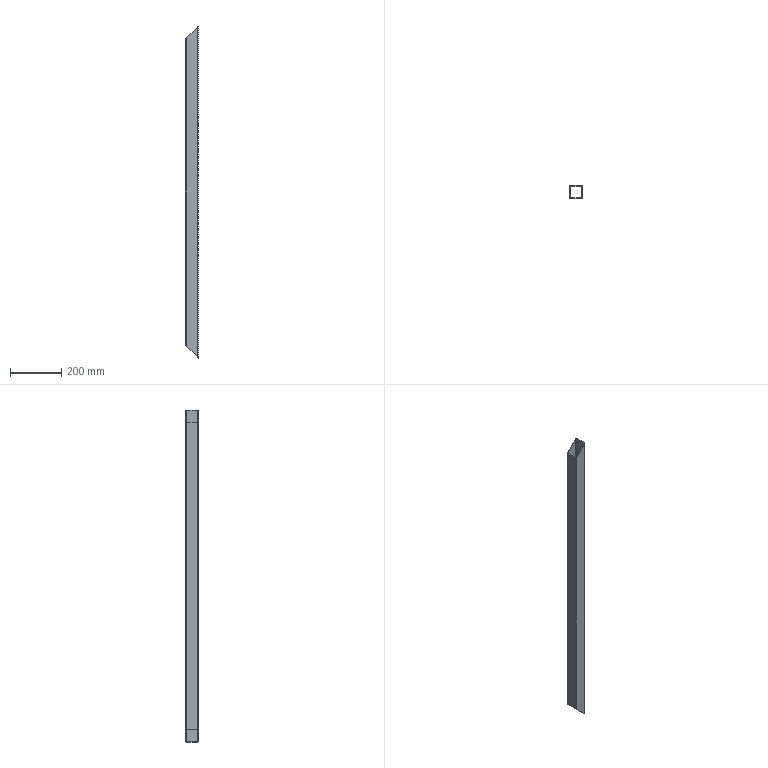Part | SolidWorks | features BaseBody 1 | 1 solid | 18 faces | box 50 x 50 x 1296 mm | volume 465629 mm3 | plane 10 | cylinder 8 | commonest cylinder face diameters 4 x4 8 x4
STEP:
#1=CARTESIAN_POINT('',(-23.,21.,600.));
#2=VERTEX_POINT('',#1);
#3=CARTESIAN_POINT('',(-23.,-21.,600.));
#4=VERTEX_POINT('',#3);
#5=CARTESIAN_POINT('',(-23.,21.,600.));
#6=DIRECTION('',(0.,-1.,0.));
#7=VECTOR('',#6,1000.);
#8=LINE('',#5,#7);
#9=EDGE_CURVE('',#2,#4,#8,.T.);
#10=ORIENTED_EDGE('',*,*,#9,.F.);
#11=CARTESIAN_POINT('',(-21.,23.,602.));
#12=VERTEX_POINT('',#11);
#13=CARTESIAN_POINT('',(-21.,23.,602.));
#14=CARTESIAN_POINT('',(-22.172,23.,600.828));
#15=CARTESIAN_POINT('',(-23.,22.172,600.));
#16=CARTESIAN_POINT('',(-23.,21.,600.));
#17=(BOUNDED_CURVE()B_SPLINE_CURVE(3,(#13,#14,#15,#16),.UNSPECIFIED.,.F.,.F.)B_SPLINE_CURVE_WITH_KNOTS((4,4),(4.712,6.283),.UNSPECIFIED.)CURVE()GEOMETRIC_REPRESENTATION_ITEM()RATIONAL_B_SPLINE_CURVE((1.,0.8047,0.8047,1.))REPRESENTATION_ITEM(''));
#18=EDGE_CURVE('',#12,#2,#17,.T.);
#19=ORIENTED_EDGE('',*,*,#18,.F.);
#20=CARTESIAN_POINT('',(21.,23.,644.));
#21=VERTEX_POINT('',#20);
#22=CARTESIAN_POINT('',(2.,23.,625.));
#23=DIRECTION('',(-0.7071,0.,-0.7071));
#24=VECTOR('',#23,1000.);
#25=LINE('',#22,#24);
#26=EDGE_CURVE('',#21,#12,#25,.T.);
#27=ORIENTED_EDGE('',*,*,#26,.F.);
#28=CARTESIAN_POINT('',(23.,21.,646.));
#29=VERTEX_POINT('',#28);
#30=CARTESIAN_POINT('',(23.,21.,646.));
#31=CARTESIAN_POINT('',(23.,22.172,646.));
#32=CARTESIAN_POINT('',(22.172,23.,645.172));
#33=CARTESIAN_POINT('',(21.,23.,644.));
#34=(BOUNDED_CURVE()B_SPLINE_CURVE(3,(#30,#31,#32,#33),.UNSPECIFIED.,.F.,.F.)B_SPLINE_CURVE_WITH_KNOTS((4,4),(3.142,4.712),.UNSPECIFIED.)CURVE()GEOMETRIC_REPRESENTATION_ITEM()RATIONAL_B_SPLINE_CURVE((1.,0.8047,0.8047,1.))REPRESENTATION_ITEM(''));
#35=EDGE_CURVE('',#29,#21,#34,.T.);
#36=ORIENTED_EDGE('',*,*,#35,.F.);
#37=CARTESIAN_POINT('',(23.,-21.,646.));
#38=VERTEX_POINT('',#37);
#39=CARTESIAN_POINT('',(23.,21.,646.));
#40=DIRECTION('',(0.,1.,0.));
#41=VECTOR('',#40,1000.);
#42=LINE('',#39,#41);
#43=EDGE_CURVE('',#38,#29,#42,.T.);
#44=ORIENTED_EDGE('',*,*,#43,.F.);
#45=CARTESIAN_POINT('',(21.,-23.,644.));
#46=VERTEX_POINT('',#45);
#47=CARTESIAN_POINT('',(21.,-23.,644.));
#48=CARTESIAN_POINT('',(22.172,-23.,645.172));
#49=CARTESIAN_POINT('',(23.,-22.172,646.));
#50=CARTESIAN_POINT('',(23.,-21.,646.));
#51=(BOUNDED_CURVE()B_SPLINE_CURVE(3,(#47,#48,#49,#50),.UNSPECIFIED.,.F.,.F.)B_SPLINE_CURVE_WITH_KNOTS((4,4),(1.571,3.142),.UNSPECIFIED.)CURVE()GEOMETRIC_REPRESENTATION_ITEM()RATIONAL_B_SPLINE_CURVE((1.,0.8047,0.8047,1.))REPRESENTATION_ITEM(''));
#52=EDGE_CURVE('',#46,#38,#51,.T.);
#53=ORIENTED_EDGE('',*,*,#52,.F.);
#54=CARTESIAN_POINT('',(-21.,-23.,602.));
#55=VERTEX_POINT('',#54);
#56=CARTESIAN_POINT('',(2.,-23.,625.));
#57=DIRECTION('',(0.7071,0.,0.7071));
#58=VECTOR('',#57,1000.);
#59=LINE('',#56,#58);
#60=EDGE_CURVE('',#55,#46,#59,.T.);
#61=ORIENTED_EDGE('',*,*,#60,.F.);
#62=CARTESIAN_POINT('',(-23.,-21.,600.));
#63=CARTESIAN_POINT('',(-23.,-22.172,600.));
#64=CARTESIAN_POINT('',(-22.172,-23.,600.828));
#65=CARTESIAN_POINT('',(-21.,-23.,602.));
#66=(BOUNDED_CURVE()B_SPLINE_CURVE(3,(#62,#63,#64,#65),.UNSPECIFIED.,.F.,.F.)B_SPLINE_CURVE_WITH_KNOTS((4,4),(0.,1.571),.UNSPECIFIED.)CURVE()GEOMETRIC_REPRESENTATION_ITEM()RATIONAL_B_SPLINE_CURVE((1.,0.8047,0.8047,1.))REPRESENTATION_ITEM(''));
#67=EDGE_CURVE('',#4,#55,#66,.T.);
#68=ORIENTED_EDGE('',*,*,#67,.F.);
#69=EDGE_LOOP('',(#10,#19,#27,#36,#44,#53,#61,#68));
#70=FACE_BOUND('',#69,.T.);
#71=CARTESIAN_POINT('',(-25.,-21.,598.));
#72=VERTEX_POINT('',#71);
#73=CARTESIAN_POINT('',(-21.,-25.,602.));
#74=VERTEX_POINT('',#73);
#75=CARTESIAN_POINT('',(-25.,-21.,598.));
#76=CARTESIAN_POINT('',(-25.,-23.343,598.));
#77=CARTESIAN_POINT('',(-23.343,-25.,599.657));
#78=CARTESIAN_POINT('',(-21.,-25.,602.));
#79=(BOUNDED_CURVE()B_SPLINE_CURVE(3,(#75,#76,#77,#78),.UNSPECIFIED.,.F.,.F.)B_SPLINE_CURVE_WITH_KNOTS((4,4),(0.,1.571),.UNSPECIFIED.)CURVE()GEOMETRIC_REPRESENTATION_ITEM()RATIONAL_B_SPLINE_CURVE((1.,0.8047,0.8047,1.))REPRESENTATION_ITEM(''));
#80=EDGE_CURVE('',#72,#74,#79,.T.);
#81=ORIENTED_EDGE('',*,*,#80,.T.);
#82=CARTESIAN_POINT('',(21.,-25.,644.));
#83=VERTEX_POINT('',#82);
#84=CARTESIAN_POINT('',(25.,-25.,648.));
#85=DIRECTION('',(0.7071,0.,0.7071));
#86=VECTOR('',#85,1000.);
#87=LINE('',#84,#86);
#88=EDGE_CURVE('',#74,#83,#87,.T.);
#89=ORIENTED_EDGE('',*,*,#88,.T.);
#90=CARTESIAN_POINT('',(25.,-21.,648.));
#91=VERTEX_POINT('',#90);
#92=CARTESIAN_POINT('',(21.,-25.,644.));
#93=CARTESIAN_POINT('',(23.343,-25.,646.343));
#94=CARTESIAN_POINT('',(25.,-23.343,648.));
#95=CARTESIAN_POINT('',(25.,-21.,648.));
#96=(BOUNDED_CURVE()B_SPLINE_CURVE(3,(#92,#93,#94,#95),.UNSPECIFIED.,.F.,.F.)B_SPLINE_CURVE_WITH_KNOTS((4,4),(1.571,3.142),.UNSPECIFIED.)CURVE()GEOMETRIC_REPRESENTATION_ITEM()RATIONAL_B_SPLINE_CURVE((1.,0.8047,0.8047,1.))REPRESENTATION_ITEM(''));
#97=EDGE_CURVE('',#83,#91,#96,.T.);
#98=ORIENTED_EDGE('',*,*,#97,.T.);
#99=CARTESIAN_POINT('',(25.,21.,648.));
#100=VERTEX_POINT('',#99);
#101=CARTESIAN_POINT('',(25.,21.,648.));
#102=DIRECTION('',(0.,1.,0.));
#103=VECTOR('',#102,1000.);
#104=LINE('',#101,#103);
#105=EDGE_CURVE('',#91,#100,#104,.T.);
#106=ORIENTED_EDGE('',*,*,#105,.T.);
#107=CARTESIAN_POINT('',(21.,25.,644.));
#108=VERTEX_POINT('',#107);
#109=CARTESIAN_POINT('',(25.,21.,648.));
#110=CARTESIAN_POINT('',(25.,23.343,648.));
#111=CARTESIAN_POINT('',(23.343,25.,646.343));
#112=CARTESIAN_POINT('',(21.,25.,644.));
#113=(BOUNDED_CURVE()B_SPLINE_CURVE(3,(#109,#110,#111,#112),.UNSPECIFIED.,.F.,.F.)B_SPLINE_CURVE_WITH_KNOTS((4,4),(3.142,4.712),.UNSPECIFIED.)CURVE()GEOMETRIC_REPRESENTATION_ITEM()RATIONAL_B_SPLINE_CURVE((1.,0.8047,0.8047,1.))REPRESENTATION_ITEM(''));
#114=EDGE_CURVE('',#100,#108,#113,.T.);
#115=ORIENTED_EDGE('',*,*,#114,.T.);
#116=CARTESIAN_POINT('',(-21.,25.,602.));
#117=VERTEX_POINT('',#116);
#118=CARTESIAN_POINT('',(25.,25.,648.));
#119=DIRECTION('',(0.7071,0.,0.7071));
#120=VECTOR('',#119,1000.);
#121=LINE('',#118,#120);
#122=EDGE_CURVE('',#117,#108,#121,.T.);
#123=ORIENTED_EDGE('',*,*,#122,.F.);
#124=CARTESIAN_POINT('',(-25.,21.,598.));
#125=VERTEX_POINT('',#124);
#126=CARTESIAN_POINT('',(-21.,25.,602.));
#127=CARTESIAN_POINT('',(-23.343,25.,599.657));
#128=CARTESIAN_POINT('',(-25.,23.343,598.));
#129=CARTESIAN_POINT('',(-25.,21.,598.));
#130=(BOUNDED_CURVE()B_SPLINE_CURVE(3,(#126,#127,#128,#129),.UNSPECIFIED.,.F.,.F.)B_SPLINE_CURVE_WITH_KNOTS((4,4),(4.712,6.283),.UNSPECIFIED.)CURVE()GEOMETRIC_REPRESENTATION_ITEM()RATIONAL_B_SPLINE_CURVE((1.,0.8047,0.8047,1.))REPRESENTATION_ITEM(''));
#131=EDGE_CURVE('',#117,#125,#130,.T.);
#132=ORIENTED_EDGE('',*,*,#131,.T.);
#133=CARTESIAN_POINT('',(-25.,-25.,598.));
#134=DIRECTION('',(0.,1.,0.));
#135=VECTOR('',#134,1000.);
#136=LINE('',#133,#135);
#137=EDGE_CURVE('',#72,#125,#136,.T.);
#138=ORIENTED_EDGE('',*,*,#137,.F.);
#139=EDGE_LOOP('',(#81,#89,#98,#106,#115,#123,#132,#138));
#140=FACE_OUTER_BOUND('',#139,.T.);
#141=CARTESIAN_POINT('',(25.,-25.,648.));
#142=DIRECTION('',(-0.7071,0.,0.7071));
#143=DIRECTION('',(0.,1.,0.));
#144=AXIS2_PLACEMENT_3D('',#141,#142,#143);
#145=PLANE('',#144);
#146=ADVANCED_FACE('',(#70,#140),#145,.T.);
#147=CARTESIAN_POINT('',(-23.,-21.,-600.));
#148=VERTEX_POINT('',#147);
#149=CARTESIAN_POINT('',(-21.,-23.,-602.));
#150=VERTEX_POINT('',#149);
#151=CARTESIAN_POINT('',(-23.,-21.,-600.));
#152=CARTESIAN_POINT('',(-23.,-22.172,-600.));
#153=CARTESIAN_POINT('',(-22.172,-23.,-600.828));
#154=CARTESIAN_POINT('',(-21.,-23.,-602.));
#155=(BOUNDED_CURVE()B_SPLINE_CURVE(3,(#151,#152,#153,#154),.UNSPECIFIED.,.F.,.F.)B_SPLINE_CURVE_WITH_KNOTS((4,4),(3.142,4.712),.UNSPECIFIED.)CURVE()GEOMETRIC_REPRESENTATION_ITEM()RATIONAL_B_SPLINE_CURVE((1.,0.8047,0.8047,1.))REPRESENTATION_ITEM(''));
#156=EDGE_CURVE('',#148,#150,#155,.T.);
#157=ORIENTED_EDGE('',*,*,#156,.T.);
#158=CARTESIAN_POINT('',(21.,-23.,-644.));
#159=VERTEX_POINT('',#158);
#160=CARTESIAN_POINT('',(-646.,-23.,23.));
#161=DIRECTION('',(0.7071,0.,-0.7071));
#162=VECTOR('',#161,1000.);
#163=LINE('',#160,#162);
#164=EDGE_CURVE('',#150,#159,#163,.T.);
#165=ORIENTED_EDGE('',*,*,#164,.T.);
#166=CARTESIAN_POINT('',(23.,-21.,-646.));
#167=VERTEX_POINT('',#166);
#168=CARTESIAN_POINT('',(21.,-23.,-644.));
#169=CARTESIAN_POINT('',(22.172,-23.,-645.172));
#170=CARTESIAN_POINT('',(23.,-22.172,-646.));
#171=CARTESIAN_POINT('',(23.,-21.,-646.));
#172=(BOUNDED_CURVE()B_SPLINE_CURVE(3,(#168,#169,#170,#171),.UNSPECIFIED.,.F.,.F.)B_SPLINE_CURVE_WITH_KNOTS((4,4),(4.712,6.283),.UNSPECIFIED.)CURVE()GEOMETRIC_REPRESENTATION_ITEM()RATIONAL_B_SPLINE_CURVE((1.,0.8047,0.8047,1.))REPRESENTATION_ITEM(''));
#173=EDGE_CURVE('',#159,#167,#172,.T.);
#174=ORIENTED_EDGE('',*,*,#173,.T.);
#175=CARTESIAN_POINT('',(23.,21.,-646.));
#176=VERTEX_POINT('',#175);
#177=CARTESIAN_POINT('',(23.,21.,-646.));
#178=DIRECTION('',(0.,1.,0.));
#179=VECTOR('',#178,1000.);
#180=LINE('',#177,#179);
#181=EDGE_CURVE('',#167,#176,#180,.T.);
#182=ORIENTED_EDGE('',*,*,#181,.T.);
#183=CARTESIAN_POINT('',(21.,23.,-644.));
#184=VERTEX_POINT('',#183);
#185=CARTESIAN_POINT('',(23.,21.,-646.));
#186=CARTESIAN_POINT('',(23.,22.172,-646.));
#187=CARTESIAN_POINT('',(22.172,23.,-645.172));
#188=CARTESIAN_POINT('',(21.,23.,-644.));
#189=(BOUNDED_CURVE()B_SPLINE_CURVE(3,(#185,#186,#187,#188),.UNSPECIFIED.,.F.,.F.)B_SPLINE_CURVE_WITH_KNOTS((4,4),(0.,1.571),.UNSPECIFIED.)CURVE()GEOMETRIC_REPRESENTATION_ITEM()RATIONAL_B_SPLINE_CURVE((1.,0.8047,0.8047,1.))REPRESENTATION_ITEM(''));
#190=EDGE_CURVE('',#176,#184,#189,.T.);
#191=ORIENTED_EDGE('',*,*,#190,.T.);
#192=CARTESIAN_POINT('',(-21.,23.,-602.));
#193=VERTEX_POINT('',#192);
#194=CARTESIAN_POINT('',(-646.,23.,23.));
#195=DIRECTION('',(-0.7071,0.,0.7071));
#196=VECTOR('',#195,1000.);
#197=LINE('',#194,#196);
#198=EDGE_CURVE('',#184,#193,#197,.T.);
#199=ORIENTED_EDGE('',*,*,#198,.T.);
#200=CARTESIAN_POINT('',(-23.,21.,-600.));
#201=VERTEX_POINT('',#200);
#202=CARTESIAN_POINT('',(-21.,23.,-602.));
#203=CARTESIAN_POINT('',(-22.172,23.,-600.828));
#204=CARTESIAN_POINT('',(-23.,22.172,-600.));
#205=CARTESIAN_POINT('',(-23.,21.,-600.));
#206=(BOUNDED_CURVE()B_SPLINE_CURVE(3,(#202,#203,#204,#205),.UNSPECIFIED.,.F.,.F.)B_SPLINE_CURVE_WITH_KNOTS((4,4),(1.571,3.142),.UNSPECIFIED.)CURVE()GEOMETRIC_REPRESENTATION_ITEM()RATIONAL_B_SPLINE_CURVE((1.,0.8047,0.8047,1.))REPRESENTATION_ITEM(''));
#207=EDGE_CURVE('',#193,#201,#206,.T.);
#208=ORIENTED_EDGE('',*,*,#207,.T.);
#209=CARTESIAN_POINT('',(-23.,21.,-600.));
#210=DIRECTION('',(0.,-1.,0.));
#211=VECTOR('',#210,1000.);
#212=LINE('',#209,#211);
#213=EDGE_CURVE('',#201,#148,#212,.T.);
#214=ORIENTED_EDGE('',*,*,#213,.T.);
#215=EDGE_LOOP('',(#157,#165,#174,#182,#191,#199,#208,#214));
#216=FACE_BOUND('',#215,.T.);
#217=CARTESIAN_POINT('',(-25.,-21.,-598.));
#218=VERTEX_POINT('',#217);
#219=CARTESIAN_POINT('',(-25.,21.,-598.));
#220=VERTEX_POINT('',#219);
#221=CARTESIAN_POINT('',(-25.,-25.,-598.));
#222=DIRECTION('',(0.,1.,0.));
#223=VECTOR('',#222,1000.);
#224=LINE('',#221,#223);
#225=EDGE_CURVE('',#218,#220,#224,.T.);
#226=ORIENTED_EDGE('',*,*,#225,.T.);
#227=CARTESIAN_POINT('',(-21.,25.,-602.));
#228=VERTEX_POINT('',#227);
#229=CARTESIAN_POINT('',(-21.,25.,-602.));
#230=CARTESIAN_POINT('',(-23.343,25.,-599.657));
#231=CARTESIAN_POINT('',(-25.,23.343,-598.));
#232=CARTESIAN_POINT('',(-25.,21.,-598.));
#233=(BOUNDED_CURVE()B_SPLINE_CURVE(3,(#229,#230,#231,#232),.UNSPECIFIED.,.F.,.F.)B_SPLINE_CURVE_WITH_KNOTS((4,4),(1.571,3.142),.UNSPECIFIED.)CURVE()GEOMETRIC_REPRESENTATION_ITEM()RATIONAL_B_SPLINE_CURVE((1.,0.8047,0.8047,1.))REPRESENTATION_ITEM(''));
#234=EDGE_CURVE('',#228,#220,#233,.T.);
#235=ORIENTED_EDGE('',*,*,#234,.F.);
#236=CARTESIAN_POINT('',(21.,25.,-644.));
#237=VERTEX_POINT('',#236);
#238=CARTESIAN_POINT('',(25.,25.,-648.));
#239=DIRECTION('',(0.7071,0.,-0.7071));
#240=VECTOR('',#239,1000.);
#241=LINE('',#238,#240);
#242=EDGE_CURVE('',#228,#237,#241,.T.);
#243=ORIENTED_EDGE('',*,*,#242,.T.);
#244=CARTESIAN_POINT('',(25.,21.,-648.));
#245=VERTEX_POINT('',#244);
#246=CARTESIAN_POINT('',(25.,21.,-648.));
#247=CARTESIAN_POINT('',(25.,23.343,-648.));
#248=CARTESIAN_POINT('',(23.343,25.,-646.343));
#249=CARTESIAN_POINT('',(21.,25.,-644.));
#250=(BOUNDED_CURVE()B_SPLINE_CURVE(3,(#246,#247,#248,#249),.UNSPECIFIED.,.F.,.F.)B_SPLINE_CURVE_WITH_KNOTS((4,4),(0.,1.571),.UNSPECIFIED.)CURVE()GEOMETRIC_REPRESENTATION_ITEM()RATIONAL_B_SPLINE_CURVE((1.,0.8047,0.8047,1.))REPRESENTATION_ITEM(''));
#251=EDGE_CURVE('',#245,#237,#250,.T.);
#252=ORIENTED_EDGE('',*,*,#251,.F.);
#253=CARTESIAN_POINT('',(25.,-21.,-648.));
#254=VERTEX_POINT('',#253);
#255=CARTESIAN_POINT('',(25.,21.,-648.));
#256=DIRECTION('',(0.,1.,0.));
#257=VECTOR('',#256,1000.);
#258=LINE('',#255,#257);
#259=EDGE_CURVE('',#254,#245,#258,.T.);
#260=ORIENTED_EDGE('',*,*,#259,.F.);
#261=CARTESIAN_POINT('',(21.,-25.,-644.));
#262=VERTEX_POINT('',#261);
#263=CARTESIAN_POINT('',(21.,-25.,-644.));
#264=CARTESIAN_POINT('',(23.343,-25.,-646.343));
#265=CARTESIAN_POINT('',(25.,-23.343,-648.));
#266=CARTESIAN_POINT('',(25.,-21.,-648.));
#267=(BOUNDED_CURVE()B_SPLINE_CURVE(3,(#263,#264,#265,#266),.UNSPECIFIED.,.F.,.F.)B_SPLINE_CURVE_WITH_KNOTS((4,4),(4.712,6.283),.UNSPECIFIED.)CURVE()GEOMETRIC_REPRESENTATION_ITEM()RATIONAL_B_SPLINE_CURVE((1.,0.8047,0.8047,1.))REPRESENTATION_ITEM(''));
#268=EDGE_CURVE('',#262,#254,#267,.T.);
#269=ORIENTED_EDGE('',*,*,#268,.F.);
#270=CARTESIAN_POINT('',(-21.,-25.,-602.));
#271=VERTEX_POINT('',#270);
#272=CARTESIAN_POINT('',(25.,-25.,-648.));
#273=DIRECTION('',(0.7071,0.,-0.7071));
#274=VECTOR('',#273,1000.);
#275=LINE('',#272,#274);
#276=EDGE_CURVE('',#271,#262,#275,.T.);
#277=ORIENTED_EDGE('',*,*,#276,.F.);
#278=CARTESIAN_POINT('',(-25.,-21.,-598.));
#279=CARTESIAN_POINT('',(-25.,-23.343,-598.));
#280=CARTESIAN_POINT('',(-23.343,-25.,-599.657));
#281=CARTESIAN_POINT('',(-21.,-25.,-602.));
#282=(BOUNDED_CURVE()B_SPLINE_CURVE(3,(#278,#279,#280,#281),.UNSPECIFIED.,.F.,.F.)B_SPLINE_CURVE_WITH_KNOTS((4,4),(3.142,4.712),.UNSPECIFIED.)CURVE()GEOMETRIC_REPRESENTATION_ITEM()RATIONAL_B_SPLINE_CURVE((1.,0.8047,0.8047,1.))REPRESENTATION_ITEM(''));
#283=EDGE_CURVE('',#218,#271,#282,.T.);
#284=ORIENTED_EDGE('',*,*,#283,.F.);
#285=EDGE_LOOP('',(#226,#235,#243,#252,#260,#269,#277,#284));
#286=FACE_OUTER_BOUND('',#285,.T.);
#287=CARTESIAN_POINT('',(25.,-25.,-648.));
#288=DIRECTION('',(0.7071,0.,0.7071));
#289=DIRECTION('',(0.,-1.,0.));
#290=AXIS2_PLACEMENT_3D('',#287,#288,#289);
#291=PLANE('',#290);
#292=ADVANCED_FACE('',(#216,#286),#291,.F.);
#293=ORIENTED_EDGE('',*,*,#259,.T.);
#294=CARTESIAN_POINT('',(25.,21.,648.));
#295=DIRECTION('',(0.,0.,-1.));
#296=VECTOR('',#295,1000.);
#297=LINE('',#294,#296);
#298=EDGE_CURVE('',#100,#245,#297,.T.);
#299=ORIENTED_EDGE('',*,*,#298,.F.);
#300=ORIENTED_EDGE('',*,*,#105,.F.);
#301=CARTESIAN_POINT('',(25.,-21.,648.));
#302=DIRECTION('',(0.,0.,-1.));
#303=VECTOR('',#302,1000.);
#304=LINE('',#301,#303);
#305=EDGE_CURVE('',#91,#254,#304,.T.);
#306=ORIENTED_EDGE('',*,*,#305,.T.);
#307=EDGE_LOOP('',(#293,#299,#300,#306));
#308=FACE_OUTER_BOUND('',#307,.T.);
#309=CARTESIAN_POINT('',(25.,21.,648.));
#310=DIRECTION('',(-1.,0.,0.));
#311=DIRECTION('',(0.,1.,0.));
#312=AXIS2_PLACEMENT_3D('',#309,#310,#311);
#313=PLANE('',#312);
#314=ADVANCED_FACE('',(#308),#313,.F.);
#315=CARTESIAN_POINT('',(-23.,21.,648.));
#316=DIRECTION('',(0.,0.,-1.));
#317=VECTOR('',#316,1000.);
#318=LINE('',#315,#317);
#319=EDGE_CURVE('',#2,#201,#318,.T.);
#320=ORIENTED_EDGE('',*,*,#319,.F.);
#321=ORIENTED_EDGE('',*,*,#9,.T.);
#322=CARTESIAN_POINT('',(-23.,-21.,648.));
#323=DIRECTION('',(0.,0.,-1.));
#324=VECTOR('',#323,1000.);
#325=LINE('',#322,#324);
#326=EDGE_CURVE('',#4,#148,#325,.T.);
#327=ORIENTED_EDGE('',*,*,#326,.T.);
#328=ORIENTED_EDGE('',*,*,#213,.F.);
#329=EDGE_LOOP('',(#320,#321,#327,#328));
#330=FACE_OUTER_BOUND('',#329,.T.);
#331=CARTESIAN_POINT('',(-23.,21.,648.));
#332=DIRECTION('',(1.,0.,0.));
#333=DIRECTION('',(0.,1.,0.));
#334=AXIS2_PLACEMENT_3D('',#331,#332,#333);
#335=PLANE('',#334);
#336=ADVANCED_FACE('',(#330),#335,.T.);
#337=CARTESIAN_POINT('',(-21.,23.,648.));
#338=DIRECTION('',(0.,0.,-1.));
#339=VECTOR('',#338,1000.);
#340=LINE('',#337,#339);
#341=EDGE_CURVE('',#12,#193,#340,.T.);
#342=ORIENTED_EDGE('',*,*,#341,.F.);
#343=ORIENTED_EDGE('',*,*,#18,.T.);
#344=ORIENTED_EDGE('',*,*,#319,.T.);
#345=ORIENTED_EDGE('',*,*,#207,.F.);
#346=EDGE_LOOP('',(#342,#343,#344,#345));
#347=FACE_OUTER_BOUND('',#346,.T.);
#348=CARTESIAN_POINT('',(-21.,21.,648.));
#349=DIRECTION('',(0.,0.,-1.));
#350=DIRECTION('',(-1.,0.,0.));
#351=AXIS2_PLACEMENT_3D('',#348,#349,#350);
#352=CYLINDRICAL_SURFACE('',#351,2.);
#353=ADVANCED_FACE('',(#347),#352,.F.);
#354=CARTESIAN_POINT('',(21.,23.,648.));
#355=DIRECTION('',(0.,0.,-1.));
#356=VECTOR('',#355,1000.);
#357=LINE('',#354,#356);
#358=EDGE_CURVE('',#21,#184,#357,.T.);
#359=ORIENTED_EDGE('',*,*,#358,.F.);
#360=ORIENTED_EDGE('',*,*,#26,.T.);
#361=ORIENTED_EDGE('',*,*,#341,.T.);
#362=ORIENTED_EDGE('',*,*,#198,.F.);
#363=EDGE_LOOP('',(#359,#360,#361,#362));
#364=FACE_OUTER_BOUND('',#363,.T.);
#365=CARTESIAN_POINT('',(-21.,23.,648.));
#366=DIRECTION('',(0.,-1.,0.));
#367=DIRECTION('',(0.,0.,-1.));
#368=AXIS2_PLACEMENT_3D('',#365,#366,#367);
#369=PLANE('',#368);
#370=ADVANCED_FACE('',(#364),#369,.T.);
#371=CARTESIAN_POINT('',(23.,21.,648.));
#372=DIRECTION('',(0.,0.,-1.));
#373=VECTOR('',#372,1000.);
#374=LINE('',#371,#373);
#375=EDGE_CURVE('',#29,#176,#374,.T.);
#376=ORIENTED_EDGE('',*,*,#375,.F.);
#377=ORIENTED_EDGE('',*,*,#35,.T.);
#378=ORIENTED_EDGE('',*,*,#358,.T.);
#379=ORIENTED_EDGE('',*,*,#190,.F.);
#380=EDGE_LOOP('',(#376,#377,#378,#379));
#381=FACE_OUTER_BOUND('',#380,.T.);
#382=CARTESIAN_POINT('',(21.,21.,648.));
#383=DIRECTION('',(0.,0.,-1.));
#384=DIRECTION('',(-1.,0.,0.));
#385=AXIS2_PLACEMENT_3D('',#382,#383,#384);
#386=CYLINDRICAL_SURFACE('',#385,2.);
#387=ADVANCED_FACE('',(#381),#386,.F.);
#388=CARTESIAN_POINT('',(23.,-21.,648.));
#389=DIRECTION('',(0.,0.,-1.));
#390=VECTOR('',#389,1000.);
#391=LINE('',#388,#390);
#392=EDGE_CURVE('',#38,#167,#391,.T.);
#393=ORIENTED_EDGE('',*,*,#392,.F.);
#394=ORIENTED_EDGE('',*,*,#43,.T.);
#395=ORIENTED_EDGE('',*,*,#375,.T.);
#396=ORIENTED_EDGE('',*,*,#181,.F.);
#397=EDGE_LOOP('',(#393,#394,#395,#396));
#398=FACE_OUTER_BOUND('',#397,.T.);
#399=CARTESIAN_POINT('',(23.,21.,648.));
#400=DIRECTION('',(-1.,0.,0.));
#401=DIRECTION('',(0.,1.,0.));
#402=AXIS2_PLACEMENT_3D('',#399,#400,#401);
#403=PLANE('',#402);
#404=ADVANCED_FACE('',(#398),#403,.T.);
#405=CARTESIAN_POINT('',(21.,-23.,648.));
#406=DIRECTION('',(0.,0.,-1.));
#407=VECTOR('',#406,1000.);
#408=LINE('',#405,#407);
#409=EDGE_CURVE('',#46,#159,#408,.T.);
#410=ORIENTED_EDGE('',*,*,#409,.F.);
#411=ORIENTED_EDGE('',*,*,#52,.T.);
#412=ORIENTED_EDGE('',*,*,#392,.T.);
#413=ORIENTED_EDGE('',*,*,#173,.F.);
#414=EDGE_LOOP('',(#410,#411,#412,#413));
#415=FACE_OUTER_BOUND('',#414,.T.);
#416=CARTESIAN_POINT('',(21.,-21.,648.));
#417=DIRECTION('',(0.,0.,-1.));
#418=DIRECTION('',(-1.,0.,0.));
#419=AXIS2_PLACEMENT_3D('',#416,#417,#418);
#420=CYLINDRICAL_SURFACE('',#419,2.);
#421=ADVANCED_FACE('',(#415),#420,.F.);
#422=CARTESIAN_POINT('',(-21.,-23.,648.));
#423=DIRECTION('',(0.,0.,-1.));
#424=VECTOR('',#423,1000.);
#425=LINE('',#422,#424);
#426=EDGE_CURVE('',#55,#150,#425,.T.);
#427=ORIENTED_EDGE('',*,*,#426,.F.);
#428=ORIENTED_EDGE('',*,*,#60,.T.);
#429=ORIENTED_EDGE('',*,*,#409,.T.);
#430=ORIENTED_EDGE('',*,*,#164,.F.);
#431=EDGE_LOOP('',(#427,#428,#429,#430));
#432=FACE_OUTER_BOUND('',#431,.T.);
#433=CARTESIAN_POINT('',(-21.,-23.,648.));
#434=DIRECTION('',(0.,1.,0.));
#435=DIRECTION('',(1.,0.,0.));
#436=AXIS2_PLACEMENT_3D('',#433,#434,#435);
#437=PLANE('',#436);
#438=ADVANCED_FACE('',(#432),#437,.T.);
#439=ORIENTED_EDGE('',*,*,#326,.F.);
#440=ORIENTED_EDGE('',*,*,#67,.T.);
#441=ORIENTED_EDGE('',*,*,#426,.T.);
#442=ORIENTED_EDGE('',*,*,#156,.F.);
#443=EDGE_LOOP('',(#439,#440,#441,#442));
#444=FACE_OUTER_BOUND('',#443,.T.);
#445=CARTESIAN_POINT('',(-21.,-21.,648.));
#446=DIRECTION('',(0.,0.,-1.));
#447=DIRECTION('',(-1.,0.,0.));
#448=AXIS2_PLACEMENT_3D('',#445,#446,#447);
#449=CYLINDRICAL_SURFACE('',#448,2.);
#450=ADVANCED_FACE('',(#444),#449,.F.);
#451=ORIENTED_EDGE('',*,*,#137,.T.);
#452=CARTESIAN_POINT('',(-25.,21.,648.));
#453=DIRECTION('',(0.,0.,-1.));
#454=VECTOR('',#453,1000.);
#455=LINE('',#452,#454);
#456=EDGE_CURVE('',#125,#220,#455,.T.);
#457=ORIENTED_EDGE('',*,*,#456,.T.);
#458=ORIENTED_EDGE('',*,*,#225,.F.);
#459=CARTESIAN_POINT('',(-25.,-21.,648.));
#460=DIRECTION('',(0.,0.,-1.));
#461=VECTOR('',#460,1000.);
#462=LINE('',#459,#461);
#463=EDGE_CURVE('',#72,#218,#462,.T.);
#464=ORIENTED_EDGE('',*,*,#463,.F.);
#465=EDGE_LOOP('',(#451,#457,#458,#464));
#466=FACE_OUTER_BOUND('',#465,.T.);
#467=CARTESIAN_POINT('',(-25.,21.,648.));
#468=DIRECTION('',(1.,0.,0.));
#469=DIRECTION('',(0.,1.,0.));
#470=AXIS2_PLACEMENT_3D('',#467,#468,#469);
#471=PLANE('',#470);
#472=ADVANCED_FACE('',(#466),#471,.F.);
#473=ORIENTED_EDGE('',*,*,#131,.F.);
#474=CARTESIAN_POINT('',(-21.,25.,648.));
#475=DIRECTION('',(0.,0.,-1.));
#476=VECTOR('',#475,1000.);
#477=LINE('',#474,#476);
#478=EDGE_CURVE('',#117,#228,#477,.T.);
#479=ORIENTED_EDGE('',*,*,#478,.T.);
#480=ORIENTED_EDGE('',*,*,#234,.T.);
#481=ORIENTED_EDGE('',*,*,#456,.F.);
#482=EDGE_LOOP('',(#473,#479,#480,#481));
#483=FACE_OUTER_BOUND('',#482,.T.);
#484=CARTESIAN_POINT('',(-21.,21.,648.));
#485=DIRECTION('',(0.,0.,-1.));
#486=DIRECTION('',(-1.,0.,0.));
#487=AXIS2_PLACEMENT_3D('',#484,#485,#486);
#488=CYLINDRICAL_SURFACE('',#487,4.);
#489=ADVANCED_FACE('',(#483),#488,.T.);
#490=ORIENTED_EDGE('',*,*,#122,.T.);
#491=CARTESIAN_POINT('',(21.,25.,648.));
#492=DIRECTION('',(0.,0.,-1.));
#493=VECTOR('',#492,1000.);
#494=LINE('',#491,#493);
#495=EDGE_CURVE('',#108,#237,#494,.T.);
#496=ORIENTED_EDGE('',*,*,#495,.T.);
#497=ORIENTED_EDGE('',*,*,#242,.F.);
#498=ORIENTED_EDGE('',*,*,#478,.F.);
#499=EDGE_LOOP('',(#490,#496,#497,#498));
#500=FACE_OUTER_BOUND('',#499,.T.);
#501=CARTESIAN_POINT('',(-21.,25.,648.));
#502=DIRECTION('',(0.,-1.,0.));
#503=DIRECTION('',(0.,0.,-1.));
#504=AXIS2_PLACEMENT_3D('',#501,#502,#503);
#505=PLANE('',#504);
#506=ADVANCED_FACE('',(#500),#505,.F.);
#507=ORIENTED_EDGE('',*,*,#114,.F.);
#508=ORIENTED_EDGE('',*,*,#298,.T.);
#509=ORIENTED_EDGE('',*,*,#251,.T.);
#510=ORIENTED_EDGE('',*,*,#495,.F.);
#511=EDGE_LOOP('',(#507,#508,#509,#510));
#512=FACE_OUTER_BOUND('',#511,.T.);
#513=CARTESIAN_POINT('',(21.,21.,648.));
#514=DIRECTION('',(0.,0.,-1.));
#515=DIRECTION('',(-1.,0.,0.));
#516=AXIS2_PLACEMENT_3D('',#513,#514,#515);
#517=CYLINDRICAL_SURFACE('',#516,4.);
#518=ADVANCED_FACE('',(#512),#517,.T.);
#519=ORIENTED_EDGE('',*,*,#97,.F.);
#520=CARTESIAN_POINT('',(21.,-25.,648.));
#521=DIRECTION('',(0.,0.,-1.));
#522=VECTOR('',#521,1000.);
#523=LINE('',#520,#522);
#524=EDGE_CURVE('',#83,#262,#523,.T.);
#525=ORIENTED_EDGE('',*,*,#524,.T.);
#526=ORIENTED_EDGE('',*,*,#268,.T.);
#527=ORIENTED_EDGE('',*,*,#305,.F.);
#528=EDGE_LOOP('',(#519,#525,#526,#527));
#529=FACE_OUTER_BOUND('',#528,.T.);
#530=CARTESIAN_POINT('',(21.,-21.,648.));
#531=DIRECTION('',(0.,0.,-1.));
#532=DIRECTION('',(-1.,0.,0.));
#533=AXIS2_PLACEMENT_3D('',#530,#531,#532);
#534=CYLINDRICAL_SURFACE('',#533,4.);
#535=ADVANCED_FACE('',(#529),#534,.T.);
#536=ORIENTED_EDGE('',*,*,#88,.F.);
#537=CARTESIAN_POINT('',(-21.,-25.,648.));
#538=DIRECTION('',(0.,0.,-1.));
#539=VECTOR('',#538,1000.);
#540=LINE('',#537,#539);
#541=EDGE_CURVE('',#74,#271,#540,.T.);
#542=ORIENTED_EDGE('',*,*,#541,.T.);
#543=ORIENTED_EDGE('',*,*,#276,.T.);
#544=ORIENTED_EDGE('',*,*,#524,.F.);
#545=EDGE_LOOP('',(#536,#542,#543,#544));
#546=FACE_OUTER_BOUND('',#545,.T.);
#547=CARTESIAN_POINT('',(-21.,-25.,648.));
#548=DIRECTION('',(0.,1.,0.));
#549=DIRECTION('',(1.,0.,0.));
#550=AXIS2_PLACEMENT_3D('',#547,#548,#549);
#551=PLANE('',#550);
#552=ADVANCED_FACE('',(#546),#551,.F.);
#553=ORIENTED_EDGE('',*,*,#80,.F.);
#554=ORIENTED_EDGE('',*,*,#463,.T.);
#555=ORIENTED_EDGE('',*,*,#283,.T.);
#556=ORIENTED_EDGE('',*,*,#541,.F.);
#557=EDGE_LOOP('',(#553,#554,#555,#556));
#558=FACE_OUTER_BOUND('',#557,.T.);
#559=CARTESIAN_POINT('',(-21.,-21.,648.));
#560=DIRECTION('',(0.,0.,-1.));
#561=DIRECTION('',(-1.,0.,0.));
#562=AXIS2_PLACEMENT_3D('',#559,#560,#561);
#563=CYLINDRICAL_SURFACE('',#562,4.);
#564=ADVANCED_FACE('',(#558),#563,.T.);
#565=CLOSED_SHELL('',(#146,#292,#314,#336,#353,#370,#387,#404,#421,#438,#450,#472,#489,#506,#518,#535,#552,#564));
#566=MANIFOLD_SOLID_BREP('',#565);
#567=CARTESIAN_POINT('',(0.,0.,0.));
#568=DIRECTION('',(0.,0.,1.));
#569=DIRECTION('',(1.,0.,0.));
#570=AXIS2_PLACEMENT_3D('',#567,#568,#569);
#571=(LENGTH_UNIT()NAMED_UNIT(*)SI_UNIT(.MILLI.,.METRE.));
#572=UNCERTAINTY_MEASURE_WITH_UNIT(LENGTH_MEASURE(0.00001),#571,'','');
#573=(NAMED_UNIT(*)PLANE_ANGLE_UNIT()SI_UNIT($,.RADIAN.));
#574=(NAMED_UNIT(*)SI_UNIT($,.STERADIAN.)SOLID_ANGLE_UNIT());
#575=(GEOMETRIC_REPRESENTATION_CONTEXT(3)GLOBAL_UNCERTAINTY_ASSIGNED_CONTEXT((#572))GLOBAL_UNIT_ASSIGNED_CONTEXT((#571,#573,#574))REPRESENTATION_CONTEXT('',''));
#576=ADVANCED_BREP_SHAPE_REPRESENTATION('',(#566,#570),#575);